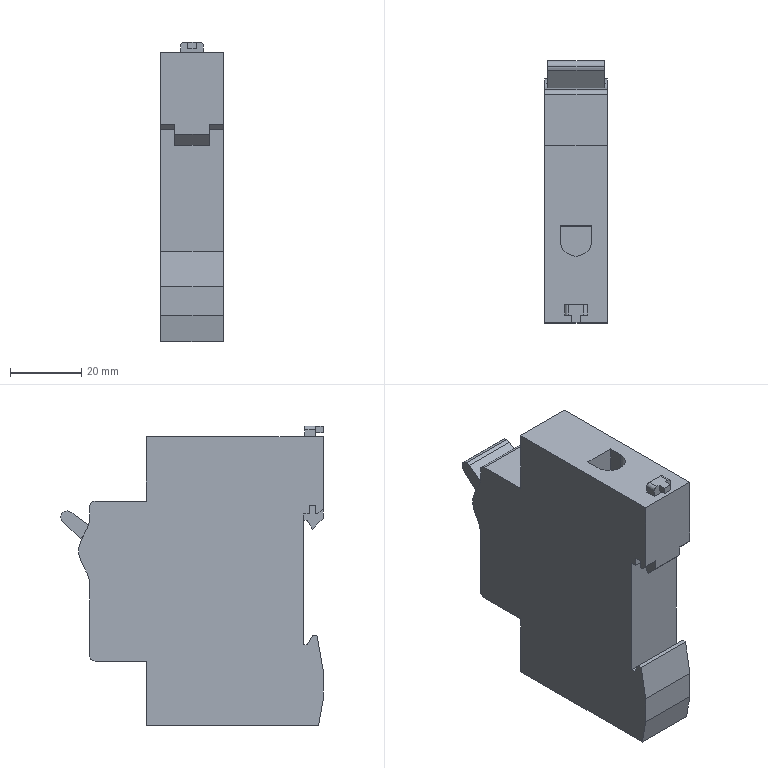Part | SolidWorks | features BaseBody 1 | 1 solid | 99 faces | box 17.6 x 73.879 x 84.3 mm | volume 78894 mm3 | plane 82 | cylinder 17 | commonest cylinder face diameters 7 x4 9 x4 2 x2 3 x2 3.6 x2 20 x2